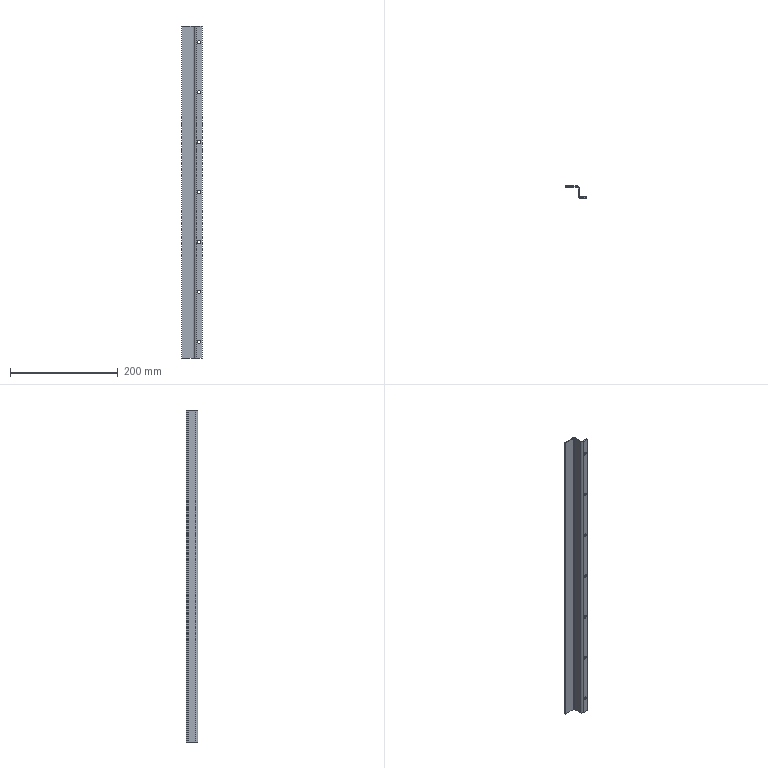Part | NX | features solid 2 | 1 solid | 28 faces | box 38 x 22 x 617 mm | volume 67998 mm3 | cylinder 18 | plane 10 | commonest cylinder face diameters 6 x14 4 x2 8 x2
STEP:
#1=CARTESIAN_POINT('',(1011.,-1578.,925.));
#2=VERTEX_POINT('',#1);
#3=CARTESIAN_POINT('',(1011.,-1576.,925.));
#4=VERTEX_POINT('',#3);
#5=CARTESIAN_POINT('',(1011.,-2194.56,925.));
#6=DIRECTION('',(0.,1.,0.));
#7=VECTOR('',#6,1000.);
#8=LINE('',#5,#7);
#9=EDGE_CURVE('',#2,#4,#8,.T.);
#10=ORIENTED_EDGE('',*,*,#9,.F.);
#11=CARTESIAN_POINT('',(1017.,-1578.,925.));
#12=VERTEX_POINT('',#11);
#13=CARTESIAN_POINT('',(1014.,-1578.,925.));
#14=DIRECTION('',(0.,1.,0.));
#15=DIRECTION('',(1.,0.,0.));
#16=AXIS2_PLACEMENT_3D('',#13,#14,#15);
#17=CIRCLE('',#16,3.);
#18=EDGE_CURVE('',#12,#2,#17,.T.);
#19=ORIENTED_EDGE('',*,*,#18,.F.);
#20=CARTESIAN_POINT('',(1017.,-1576.,925.));
#21=VERTEX_POINT('',#20);
#22=CARTESIAN_POINT('',(1017.,-2194.56,925.));
#23=DIRECTION('',(0.,1.,0.));
#24=VECTOR('',#23,1000.);
#25=LINE('',#22,#24);
#26=EDGE_CURVE('',#21,#12,#25,.F.);
#27=ORIENTED_EDGE('',*,*,#26,.F.);
#28=CARTESIAN_POINT('',(1014.,-1576.,925.));
#29=DIRECTION('',(0.,1.,0.));
#30=DIRECTION('',(0.,0.,1.));
#31=AXIS2_PLACEMENT_3D('',#28,#29,#30);
#32=CIRCLE('',#31,3.);
#33=EDGE_CURVE('',#21,#4,#32,.T.);
#34=ORIENTED_EDGE('',*,*,#33,.T.);
#35=EDGE_LOOP('',(#10,#19,#27,#34));
#36=FACE_BOUND('',#35,.T.);
#37=CARTESIAN_POINT('',(1014.,-2194.56,925.));
#38=DIRECTION('',(0.,1.,0.));
#39=DIRECTION('',(1.,0.,0.));
#40=AXIS2_PLACEMENT_3D('',#37,#38,#39);
#41=CYLINDRICAL_SURFACE('',#40,3.);
#42=ADVANCED_FACE('',(#36),#41,.F.);
#43=CARTESIAN_POINT('',(1011.,-1578.,832.167));
#44=VERTEX_POINT('',#43);
#45=CARTESIAN_POINT('',(1011.,-1576.,832.167));
#46=VERTEX_POINT('',#45);
#47=CARTESIAN_POINT('',(1011.,-2194.56,832.167));
#48=DIRECTION('',(0.,1.,0.));
#49=VECTOR('',#48,1000.);
#50=LINE('',#47,#49);
#51=EDGE_CURVE('',#44,#46,#50,.T.);
#52=ORIENTED_EDGE('',*,*,#51,.F.);
#53=CARTESIAN_POINT('',(1017.,-1578.,832.167));
#54=VERTEX_POINT('',#53);
#55=CARTESIAN_POINT('',(1014.,-1578.,832.167));
#56=DIRECTION('',(0.,1.,0.));
#57=DIRECTION('',(1.,0.,0.));
#58=AXIS2_PLACEMENT_3D('',#55,#56,#57);
#59=CIRCLE('',#58,3.);
#60=EDGE_CURVE('',#54,#44,#59,.T.);
#61=ORIENTED_EDGE('',*,*,#60,.F.);
#62=CARTESIAN_POINT('',(1017.,-1576.,832.167));
#63=VERTEX_POINT('',#62);
#64=CARTESIAN_POINT('',(1017.,-2194.56,832.167));
#65=DIRECTION('',(0.,1.,0.));
#66=VECTOR('',#65,1000.);
#67=LINE('',#64,#66);
#68=EDGE_CURVE('',#63,#54,#67,.F.);
#69=ORIENTED_EDGE('',*,*,#68,.F.);
#70=CARTESIAN_POINT('',(1014.,-1576.,832.167));
#71=DIRECTION('',(0.,1.,0.));
#72=DIRECTION('',(0.,0.,1.));
#73=AXIS2_PLACEMENT_3D('',#70,#71,#72);
#74=CIRCLE('',#73,3.);
#75=EDGE_CURVE('',#63,#46,#74,.T.);
#76=ORIENTED_EDGE('',*,*,#75,.T.);
#77=EDGE_LOOP('',(#52,#61,#69,#76));
#78=FACE_BOUND('',#77,.T.);
#79=CARTESIAN_POINT('',(1014.,-2194.56,832.167));
#80=DIRECTION('',(0.,1.,0.));
#81=DIRECTION('',(1.,0.,0.));
#82=AXIS2_PLACEMENT_3D('',#79,#80,#81);
#83=CYLINDRICAL_SURFACE('',#82,3.);
#84=ADVANCED_FACE('',(#78),#83,.F.);
#85=CARTESIAN_POINT('',(1011.,-1576.,739.333));
#86=VERTEX_POINT('',#85);
#87=CARTESIAN_POINT('',(1011.,-1578.,739.333));
#88=VERTEX_POINT('',#87);
#89=CARTESIAN_POINT('',(1011.,-2194.56,739.333));
#90=DIRECTION('',(0.,1.,0.));
#91=VECTOR('',#90,1000.);
#92=LINE('',#89,#91);
#93=EDGE_CURVE('',#86,#88,#92,.F.);
#94=ORIENTED_EDGE('',*,*,#93,.T.);
#95=CARTESIAN_POINT('',(1017.,-1578.,739.333));
#96=VERTEX_POINT('',#95);
#97=CARTESIAN_POINT('',(1014.,-1578.,739.333));
#98=DIRECTION('',(0.,1.,0.));
#99=DIRECTION('',(1.,0.,0.));
#100=AXIS2_PLACEMENT_3D('',#97,#98,#99);
#101=CIRCLE('',#100,3.);
#102=EDGE_CURVE('',#96,#88,#101,.T.);
#103=ORIENTED_EDGE('',*,*,#102,.F.);
#104=CARTESIAN_POINT('',(1017.,-1576.,739.333));
#105=VERTEX_POINT('',#104);
#106=CARTESIAN_POINT('',(1017.,-2194.56,739.333));
#107=DIRECTION('',(0.,1.,0.));
#108=VECTOR('',#107,1000.);
#109=LINE('',#106,#108);
#110=EDGE_CURVE('',#96,#105,#109,.T.);
#111=ORIENTED_EDGE('',*,*,#110,.T.);
#112=CARTESIAN_POINT('',(1014.,-1576.,739.333));
#113=DIRECTION('',(0.,1.,0.));
#114=DIRECTION('',(0.,0.,1.));
#115=AXIS2_PLACEMENT_3D('',#112,#113,#114);
#116=CIRCLE('',#115,3.);
#117=EDGE_CURVE('',#105,#86,#116,.T.);
#118=ORIENTED_EDGE('',*,*,#117,.T.);
#119=EDGE_LOOP('',(#94,#103,#111,#118));
#120=FACE_BOUND('',#119,.T.);
#121=CARTESIAN_POINT('',(1014.,-2194.56,739.333));
#122=DIRECTION('',(0.,1.,0.));
#123=DIRECTION('',(1.,0.,0.));
#124=AXIS2_PLACEMENT_3D('',#121,#122,#123);
#125=CYLINDRICAL_SURFACE('',#124,3.);
#126=ADVANCED_FACE('',(#120),#125,.F.);
#127=CARTESIAN_POINT('',(1011.,-1578.,646.5));
#128=VERTEX_POINT('',#127);
#129=CARTESIAN_POINT('',(1011.,-1576.,646.5));
#130=VERTEX_POINT('',#129);
#131=CARTESIAN_POINT('',(1011.,-2194.56,646.5));
#132=DIRECTION('',(0.,1.,0.));
#133=VECTOR('',#132,1000.);
#134=LINE('',#131,#133);
#135=EDGE_CURVE('',#128,#130,#134,.T.);
#136=ORIENTED_EDGE('',*,*,#135,.F.);
#137=CARTESIAN_POINT('',(1017.,-1578.,646.5));
#138=VERTEX_POINT('',#137);
#139=CARTESIAN_POINT('',(1014.,-1578.,646.5));
#140=DIRECTION('',(0.,1.,0.));
#141=DIRECTION('',(1.,0.,0.));
#142=AXIS2_PLACEMENT_3D('',#139,#140,#141);
#143=CIRCLE('',#142,3.);
#144=EDGE_CURVE('',#138,#128,#143,.T.);
#145=ORIENTED_EDGE('',*,*,#144,.F.);
#146=CARTESIAN_POINT('',(1017.,-1576.,646.5));
#147=VERTEX_POINT('',#146);
#148=CARTESIAN_POINT('',(1017.,-2194.56,646.5));
#149=DIRECTION('',(0.,1.,0.));
#150=VECTOR('',#149,1000.);
#151=LINE('',#148,#150);
#152=EDGE_CURVE('',#147,#138,#151,.F.);
#153=ORIENTED_EDGE('',*,*,#152,.F.);
#154=CARTESIAN_POINT('',(1014.,-1576.,646.5));
#155=DIRECTION('',(0.,1.,0.));
#156=DIRECTION('',(0.,0.,1.));
#157=AXIS2_PLACEMENT_3D('',#154,#155,#156);
#158=CIRCLE('',#157,3.);
#159=EDGE_CURVE('',#147,#130,#158,.T.);
#160=ORIENTED_EDGE('',*,*,#159,.T.);
#161=EDGE_LOOP('',(#136,#145,#153,#160));
#162=FACE_BOUND('',#161,.T.);
#163=CARTESIAN_POINT('',(1014.,-2194.56,646.5));
#164=DIRECTION('',(0.,1.,0.));
#165=DIRECTION('',(1.,0.,0.));
#166=AXIS2_PLACEMENT_3D('',#163,#164,#165);
#167=CYLINDRICAL_SURFACE('',#166,3.);
#168=ADVANCED_FACE('',(#162),#167,.F.);
#169=CARTESIAN_POINT('',(1011.,-1576.,553.667));
#170=VERTEX_POINT('',#169);
#171=CARTESIAN_POINT('',(1011.,-1578.,553.667));
#172=VERTEX_POINT('',#171);
#173=CARTESIAN_POINT('',(1011.,-2194.56,553.667));
#174=DIRECTION('',(0.,1.,0.));
#175=VECTOR('',#174,1000.);
#176=LINE('',#173,#175);
#177=EDGE_CURVE('',#170,#172,#176,.F.);
#178=ORIENTED_EDGE('',*,*,#177,.T.);
#179=CARTESIAN_POINT('',(1017.,-1578.,553.667));
#180=VERTEX_POINT('',#179);
#181=CARTESIAN_POINT('',(1014.,-1578.,553.667));
#182=DIRECTION('',(0.,1.,0.));
#183=DIRECTION('',(1.,0.,0.));
#184=AXIS2_PLACEMENT_3D('',#181,#182,#183);
#185=CIRCLE('',#184,3.);
#186=EDGE_CURVE('',#180,#172,#185,.T.);
#187=ORIENTED_EDGE('',*,*,#186,.F.);
#188=CARTESIAN_POINT('',(1017.,-1576.,553.667));
#189=VERTEX_POINT('',#188);
#190=CARTESIAN_POINT('',(1017.,-2194.56,553.667));
#191=DIRECTION('',(0.,1.,0.));
#192=VECTOR('',#191,1000.);
#193=LINE('',#190,#192);
#194=EDGE_CURVE('',#180,#189,#193,.T.);
#195=ORIENTED_EDGE('',*,*,#194,.T.);
#196=CARTESIAN_POINT('',(1014.,-1576.,553.667));
#197=DIRECTION('',(0.,1.,0.));
#198=DIRECTION('',(0.,0.,1.));
#199=AXIS2_PLACEMENT_3D('',#196,#197,#198);
#200=CIRCLE('',#199,3.);
#201=EDGE_CURVE('',#189,#170,#200,.T.);
#202=ORIENTED_EDGE('',*,*,#201,.T.);
#203=EDGE_LOOP('',(#178,#187,#195,#202));
#204=FACE_BOUND('',#203,.T.);
#205=CARTESIAN_POINT('',(1014.,-2194.56,553.667));
#206=DIRECTION('',(0.,1.,0.));
#207=DIRECTION('',(1.,0.,0.));
#208=AXIS2_PLACEMENT_3D('',#205,#206,#207);
#209=CYLINDRICAL_SURFACE('',#208,3.);
#210=ADVANCED_FACE('',(#204),#209,.F.);
#211=CARTESIAN_POINT('',(1011.,-1576.,460.833));
#212=VERTEX_POINT('',#211);
#213=CARTESIAN_POINT('',(1011.,-1578.,460.833));
#214=VERTEX_POINT('',#213);
#215=CARTESIAN_POINT('',(1011.,-2194.56,460.833));
#216=DIRECTION('',(0.,1.,0.));
#217=VECTOR('',#216,1000.);
#218=LINE('',#215,#217);
#219=EDGE_CURVE('',#212,#214,#218,.F.);
#220=ORIENTED_EDGE('',*,*,#219,.T.);
#221=CARTESIAN_POINT('',(1017.,-1578.,460.833));
#222=VERTEX_POINT('',#221);
#223=CARTESIAN_POINT('',(1014.,-1578.,460.833));
#224=DIRECTION('',(0.,1.,0.));
#225=DIRECTION('',(1.,0.,0.));
#226=AXIS2_PLACEMENT_3D('',#223,#224,#225);
#227=CIRCLE('',#226,3.);
#228=EDGE_CURVE('',#222,#214,#227,.T.);
#229=ORIENTED_EDGE('',*,*,#228,.F.);
#230=CARTESIAN_POINT('',(1017.,-1576.,460.833));
#231=VERTEX_POINT('',#230);
#232=CARTESIAN_POINT('',(1017.,-2194.56,460.833));
#233=DIRECTION('',(0.,1.,0.));
#234=VECTOR('',#233,1000.);
#235=LINE('',#232,#234);
#236=EDGE_CURVE('',#222,#231,#235,.T.);
#237=ORIENTED_EDGE('',*,*,#236,.T.);
#238=CARTESIAN_POINT('',(1014.,-1576.,460.833));
#239=DIRECTION('',(0.,1.,0.));
#240=DIRECTION('',(0.,0.,1.));
#241=AXIS2_PLACEMENT_3D('',#238,#239,#240);
#242=CIRCLE('',#241,3.);
#243=EDGE_CURVE('',#231,#212,#242,.T.);
#244=ORIENTED_EDGE('',*,*,#243,.T.);
#245=EDGE_LOOP('',(#220,#229,#237,#244));
#246=FACE_BOUND('',#245,.T.);
#247=CARTESIAN_POINT('',(1014.,-2194.56,460.833));
#248=DIRECTION('',(0.,1.,0.));
#249=DIRECTION('',(1.,0.,0.));
#250=AXIS2_PLACEMENT_3D('',#247,#248,#249);
#251=CYLINDRICAL_SURFACE('',#250,3.);
#252=ADVANCED_FACE('',(#246),#251,.F.);
#253=CARTESIAN_POINT('',(1011.,-1578.,368.));
#254=VERTEX_POINT('',#253);
#255=CARTESIAN_POINT('',(1011.,-1576.,368.));
#256=VERTEX_POINT('',#255);
#257=CARTESIAN_POINT('',(1011.,-2194.56,368.));
#258=DIRECTION('',(0.,1.,0.));
#259=VECTOR('',#258,1000.);
#260=LINE('',#257,#259);
#261=EDGE_CURVE('',#254,#256,#260,.T.);
#262=ORIENTED_EDGE('',*,*,#261,.F.);
#263=CARTESIAN_POINT('',(1017.,-1578.,368.));
#264=VERTEX_POINT('',#263);
#265=CARTESIAN_POINT('',(1014.,-1578.,368.));
#266=DIRECTION('',(0.,1.,0.));
#267=DIRECTION('',(1.,0.,0.));
#268=AXIS2_PLACEMENT_3D('',#265,#266,#267);
#269=CIRCLE('',#268,3.);
#270=EDGE_CURVE('',#264,#254,#269,.T.);
#271=ORIENTED_EDGE('',*,*,#270,.F.);
#272=CARTESIAN_POINT('',(1017.,-1576.,368.));
#273=VERTEX_POINT('',#272);
#274=CARTESIAN_POINT('',(1017.,-2194.56,368.));
#275=DIRECTION('',(0.,1.,0.));
#276=VECTOR('',#275,1000.);
#277=LINE('',#274,#276);
#278=EDGE_CURVE('',#273,#264,#277,.F.);
#279=ORIENTED_EDGE('',*,*,#278,.F.);
#280=CARTESIAN_POINT('',(1014.,-1576.,368.));
#281=DIRECTION('',(0.,1.,0.));
#282=DIRECTION('',(0.,0.,1.));
#283=AXIS2_PLACEMENT_3D('',#280,#281,#282);
#284=CIRCLE('',#283,3.);
#285=EDGE_CURVE('',#273,#256,#284,.T.);
#286=ORIENTED_EDGE('',*,*,#285,.T.);
#287=EDGE_LOOP('',(#262,#271,#279,#286));
#288=FACE_BOUND('',#287,.T.);
#289=CARTESIAN_POINT('',(1014.,-2194.56,368.));
#290=DIRECTION('',(0.,1.,0.));
#291=DIRECTION('',(1.,0.,0.));
#292=AXIS2_PLACEMENT_3D('',#289,#290,#291);
#293=CYLINDRICAL_SURFACE('',#292,3.);
#294=ADVANCED_FACE('',(#288),#293,.F.);
#295=CARTESIAN_POINT('',(1003.,-1558.,955.));
#296=VERTEX_POINT('',#295);
#297=CARTESIAN_POINT('',(982.,-1558.,955.));
#298=VERTEX_POINT('',#297);
#299=CARTESIAN_POINT('',(1005.,-1558.,955.));
#300=DIRECTION('',(-1.,0.,0.));
#301=VECTOR('',#300,1000.);
#302=LINE('',#299,#301);
#303=EDGE_CURVE('',#296,#298,#302,.T.);
#304=ORIENTED_EDGE('',*,*,#303,.T.);
#305=CARTESIAN_POINT('',(982.,-1558.,338.));
#306=VERTEX_POINT('',#305);
#307=CARTESIAN_POINT('',(982.,-1558.,338.));
#308=DIRECTION('',(0.,0.,1.));
#309=VECTOR('',#308,1000.);
#310=LINE('',#307,#309);
#311=EDGE_CURVE('',#306,#298,#310,.T.);
#312=ORIENTED_EDGE('',*,*,#311,.F.);
#313=CARTESIAN_POINT('',(1003.,-1558.,338.));
#314=VERTEX_POINT('',#313);
#315=CARTESIAN_POINT('',(1005.,-1558.,338.));
#316=DIRECTION('',(-1.,0.,0.));
#317=VECTOR('',#316,1000.);
#318=LINE('',#315,#317);
#319=EDGE_CURVE('',#314,#306,#318,.T.);
#320=ORIENTED_EDGE('',*,*,#319,.F.);
#321=CARTESIAN_POINT('',(1003.,-1558.,338.));
#322=DIRECTION('',(0.,0.,1.));
#323=VECTOR('',#322,1000.);
#324=LINE('',#321,#323);
#325=EDGE_CURVE('',#314,#296,#324,.T.);
#326=ORIENTED_EDGE('',*,*,#325,.T.);
#327=EDGE_LOOP('',(#304,#312,#320,#326));
#328=FACE_BOUND('',#327,.T.);
#329=CARTESIAN_POINT('',(1005.,-1558.,338.));
#330=DIRECTION('',(0.,1.,0.));
#331=DIRECTION('',(0.,0.,-1.));
#332=AXIS2_PLACEMENT_3D('',#329,#330,#331);
#333=PLANE('',#332);
#334=ADVANCED_FACE('',(#328),#333,.F.);
#335=CARTESIAN_POINT('',(1005.,-1560.,955.));
#336=VERTEX_POINT('',#335);
#337=CARTESIAN_POINT('',(1003.,-1560.,955.));
#338=DIRECTION('',(0.,0.,1.));
#339=DIRECTION('',(1.,0.,0.));
#340=AXIS2_PLACEMENT_3D('',#337,#338,#339);
#341=CIRCLE('',#340,2.);
#342=EDGE_CURVE('',#336,#296,#341,.T.);
#343=ORIENTED_EDGE('',*,*,#342,.T.);
#344=ORIENTED_EDGE('',*,*,#325,.F.);
#345=CARTESIAN_POINT('',(1005.,-1560.,338.));
#346=VERTEX_POINT('',#345);
#347=CARTESIAN_POINT('',(1003.,-1560.,338.));
#348=DIRECTION('',(0.,0.,1.));
#349=DIRECTION('',(1.,0.,0.));
#350=AXIS2_PLACEMENT_3D('',#347,#348,#349);
#351=CIRCLE('',#350,2.);
#352=EDGE_CURVE('',#346,#314,#351,.T.);
#353=ORIENTED_EDGE('',*,*,#352,.F.);
#354=CARTESIAN_POINT('',(1005.,-1560.,338.));
#355=DIRECTION('',(0.,0.,1.));
#356=VECTOR('',#355,1000.);
#357=LINE('',#354,#356);
#358=EDGE_CURVE('',#346,#336,#357,.T.);
#359=ORIENTED_EDGE('',*,*,#358,.T.);
#360=EDGE_LOOP('',(#343,#344,#353,#359));
#361=FACE_BOUND('',#360,.T.);
#362=CARTESIAN_POINT('',(1003.,-1560.,338.));
#363=DIRECTION('',(0.,0.,1.));
#364=DIRECTION('',(-1.,0.,0.));
#365=AXIS2_PLACEMENT_3D('',#362,#363,#364);
#366=CYLINDRICAL_SURFACE('',#365,2.);
#367=ADVANCED_FACE('',(#361),#366,.F.);
#368=CARTESIAN_POINT('',(1005.,-1574.,955.));
#369=VERTEX_POINT('',#368);
#370=CARTESIAN_POINT('',(1005.,-1578.,955.));
#371=DIRECTION('',(0.,1.,0.));
#372=VECTOR('',#371,1000.);
#373=LINE('',#370,#372);
#374=EDGE_CURVE('',#369,#336,#373,.T.);
#375=ORIENTED_EDGE('',*,*,#374,.T.);
#376=ORIENTED_EDGE('',*,*,#358,.F.);
#377=CARTESIAN_POINT('',(1005.,-1574.,338.));
#378=VERTEX_POINT('',#377);
#379=CARTESIAN_POINT('',(1005.,-1578.,338.));
#380=DIRECTION('',(0.,1.,0.));
#381=VECTOR('',#380,1000.);
#382=LINE('',#379,#381);
#383=EDGE_CURVE('',#378,#346,#382,.T.);
#384=ORIENTED_EDGE('',*,*,#383,.F.);
#385=CARTESIAN_POINT('',(1005.,-1574.,338.));
#386=DIRECTION('',(0.,0.,1.));
#387=VECTOR('',#386,1000.);
#388=LINE('',#385,#387);
#389=EDGE_CURVE('',#378,#369,#388,.T.);
#390=ORIENTED_EDGE('',*,*,#389,.T.);
#391=EDGE_LOOP('',(#375,#376,#384,#390));
#392=FACE_BOUND('',#391,.T.);
#393=CARTESIAN_POINT('',(1005.,-1578.,338.));
#394=DIRECTION('',(1.,0.,0.));
#395=DIRECTION('',(0.,0.,-1.));
#396=AXIS2_PLACEMENT_3D('',#393,#394,#395);
#397=PLANE('',#396);
#398=ADVANCED_FACE('',(#392),#397,.F.);
#399=CARTESIAN_POINT('',(1009.,-1578.,955.));
#400=VERTEX_POINT('',#399);
#401=CARTESIAN_POINT('',(1009.,-1574.,955.));
#402=DIRECTION('',(0.,0.,-1.));
#403=DIRECTION('',(-1.,0.,0.));
#404=AXIS2_PLACEMENT_3D('',#401,#402,#403);
#405=CIRCLE('',#404,4.);
#406=EDGE_CURVE('',#400,#369,#405,.T.);
#407=ORIENTED_EDGE('',*,*,#406,.T.);
#408=ORIENTED_EDGE('',*,*,#389,.F.);
#409=CARTESIAN_POINT('',(1009.,-1578.,338.));
#410=VERTEX_POINT('',#409);
#411=CARTESIAN_POINT('',(1009.,-1574.,338.));
#412=DIRECTION('',(0.,0.,-1.));
#413=DIRECTION('',(-1.,0.,0.));
#414=AXIS2_PLACEMENT_3D('',#411,#412,#413);
#415=CIRCLE('',#414,4.);
#416=EDGE_CURVE('',#410,#378,#415,.T.);
#417=ORIENTED_EDGE('',*,*,#416,.F.);
#418=CARTESIAN_POINT('',(1009.,-1578.,338.));
#419=DIRECTION('',(0.,0.,1.));
#420=VECTOR('',#419,1000.);
#421=LINE('',#418,#420);
#422=EDGE_CURVE('',#410,#400,#421,.T.);
#423=ORIENTED_EDGE('',*,*,#422,.T.);
#424=EDGE_LOOP('',(#407,#408,#417,#423));
#425=FACE_BOUND('',#424,.T.);
#426=CARTESIAN_POINT('',(1009.,-1574.,338.));
#427=DIRECTION('',(0.,0.,1.));
#428=DIRECTION('',(-1.,0.,0.));
#429=AXIS2_PLACEMENT_3D('',#426,#427,#428);
#430=CYLINDRICAL_SURFACE('',#429,4.);
#431=ADVANCED_FACE('',(#425),#430,.T.);
#432=ORIENTED_EDGE('',*,*,#270,.T.);
#433=CARTESIAN_POINT('',(1014.,-1578.,368.));
#434=DIRECTION('',(0.,1.,0.));
#435=DIRECTION('',(1.,0.,0.));
#436=AXIS2_PLACEMENT_3D('',#433,#434,#435);
#437=CIRCLE('',#436,3.);
#438=EDGE_CURVE('',#254,#264,#437,.T.);
#439=ORIENTED_EDGE('',*,*,#438,.T.);
#440=EDGE_LOOP('',(#432,#439));
#441=FACE_BOUND('',#440,.T.);
#442=ORIENTED_EDGE('',*,*,#228,.T.);
#443=CARTESIAN_POINT('',(1014.,-1578.,460.833));
#444=DIRECTION('',(0.,1.,0.));
#445=DIRECTION('',(1.,0.,0.));
#446=AXIS2_PLACEMENT_3D('',#443,#444,#445);
#447=CIRCLE('',#446,3.);
#448=EDGE_CURVE('',#214,#222,#447,.T.);
#449=ORIENTED_EDGE('',*,*,#448,.T.);
#450=EDGE_LOOP('',(#442,#449));
#451=FACE_BOUND('',#450,.T.);
#452=ORIENTED_EDGE('',*,*,#186,.T.);
#453=CARTESIAN_POINT('',(1014.,-1578.,553.667));
#454=DIRECTION('',(0.,1.,0.));
#455=DIRECTION('',(1.,0.,0.));
#456=AXIS2_PLACEMENT_3D('',#453,#454,#455);
#457=CIRCLE('',#456,3.);
#458=EDGE_CURVE('',#172,#180,#457,.T.);
#459=ORIENTED_EDGE('',*,*,#458,.T.);
#460=EDGE_LOOP('',(#452,#459));
#461=FACE_BOUND('',#460,.T.);
#462=ORIENTED_EDGE('',*,*,#144,.T.);
#463=CARTESIAN_POINT('',(1014.,-1578.,646.5));
#464=DIRECTION('',(0.,1.,0.));
#465=DIRECTION('',(1.,0.,0.));
#466=AXIS2_PLACEMENT_3D('',#463,#464,#465);
#467=CIRCLE('',#466,3.);
#468=EDGE_CURVE('',#128,#138,#467,.T.);
#469=ORIENTED_EDGE('',*,*,#468,.T.);
#470=EDGE_LOOP('',(#462,#469));
#471=FACE_BOUND('',#470,.T.);
#472=ORIENTED_EDGE('',*,*,#102,.T.);
#473=CARTESIAN_POINT('',(1014.,-1578.,739.333));
#474=DIRECTION('',(0.,1.,0.));
#475=DIRECTION('',(1.,0.,0.));
#476=AXIS2_PLACEMENT_3D('',#473,#474,#475);
#477=CIRCLE('',#476,3.);
#478=EDGE_CURVE('',#88,#96,#477,.T.);
#479=ORIENTED_EDGE('',*,*,#478,.T.);
#480=EDGE_LOOP('',(#472,#479));
#481=FACE_BOUND('',#480,.T.);
#482=ORIENTED_EDGE('',*,*,#60,.T.);
#483=CARTESIAN_POINT('',(1014.,-1578.,832.167));
#484=DIRECTION('',(0.,1.,0.));
#485=DIRECTION('',(1.,0.,0.));
#486=AXIS2_PLACEMENT_3D('',#483,#484,#485);
#487=CIRCLE('',#486,3.);
#488=EDGE_CURVE('',#44,#54,#487,.T.);
#489=ORIENTED_EDGE('',*,*,#488,.T.);
#490=EDGE_LOOP('',(#482,#489));
#491=FACE_BOUND('',#490,.T.);
#492=ORIENTED_EDGE('',*,*,#18,.T.);
#493=CARTESIAN_POINT('',(1014.,-1578.,925.));
#494=DIRECTION('',(0.,1.,0.));
#495=DIRECTION('',(1.,0.,0.));
#496=AXIS2_PLACEMENT_3D('',#493,#494,#495);
#497=CIRCLE('',#496,3.);
#498=EDGE_CURVE('',#2,#12,#497,.T.);
#499=ORIENTED_EDGE('',*,*,#498,.T.);
#500=EDGE_LOOP('',(#492,#499));
#501=FACE_BOUND('',#500,.T.);
#502=CARTESIAN_POINT('',(1020.,-1578.,955.));
#503=VERTEX_POINT('',#502);
#504=CARTESIAN_POINT('',(1020.,-1578.,955.));
#505=DIRECTION('',(-1.,0.,0.));
#506=VECTOR('',#505,1000.);
#507=LINE('',#504,#506);
#508=EDGE_CURVE('',#503,#400,#507,.T.);
#509=ORIENTED_EDGE('',*,*,#508,.T.);
#510=ORIENTED_EDGE('',*,*,#422,.F.);
#511=CARTESIAN_POINT('',(1020.,-1578.,338.));
#512=VERTEX_POINT('',#511);
#513=CARTESIAN_POINT('',(1020.,-1578.,338.));
#514=DIRECTION('',(-1.,0.,0.));
#515=VECTOR('',#514,1000.);
#516=LINE('',#513,#515);
#517=EDGE_CURVE('',#512,#410,#516,.T.);
#518=ORIENTED_EDGE('',*,*,#517,.F.);
#519=CARTESIAN_POINT('',(1020.,-1578.,338.));
#520=DIRECTION('',(0.,0.,1.));
#521=VECTOR('',#520,1000.);
#522=LINE('',#519,#521);
#523=EDGE_CURVE('',#512,#503,#522,.T.);
#524=ORIENTED_EDGE('',*,*,#523,.T.);
#525=EDGE_LOOP('',(#509,#510,#518,#524));
#526=FACE_BOUND('',#525,.T.);
#527=CARTESIAN_POINT('',(1020.,-1578.,338.));
#528=DIRECTION('',(0.,1.,0.));
#529=DIRECTION('',(0.,0.,-1.));
#530=AXIS2_PLACEMENT_3D('',#527,#528,#529);
#531=PLANE('',#530);
#532=ADVANCED_FACE('',(#441,#451,#461,#471,#481,#491,#501,#526),#531,.F.);
#533=CARTESIAN_POINT('',(1003.,-1556.,955.));
#534=VERTEX_POINT('',#533);
#535=CARTESIAN_POINT('',(982.,-1556.,955.));
#536=VERTEX_POINT('',#535);
#537=CARTESIAN_POINT('',(1005.,-1556.,955.));
#538=DIRECTION('',(-1.,0.,0.));
#539=VECTOR('',#538,1000.);
#540=LINE('',#537,#539);
#541=EDGE_CURVE('',#534,#536,#540,.T.);
#542=ORIENTED_EDGE('',*,*,#541,.F.);
#543=CARTESIAN_POINT('',(1003.,-1556.,338.));
#544=VERTEX_POINT('',#543);
#545=CARTESIAN_POINT('',(1003.,-1556.,338.));
#546=DIRECTION('',(0.,0.,1.));
#547=VECTOR('',#546,1000.);
#548=LINE('',#545,#547);
#549=EDGE_CURVE('',#544,#534,#548,.T.);
#550=ORIENTED_EDGE('',*,*,#549,.F.);
#551=CARTESIAN_POINT('',(982.,-1556.,338.));
#552=VERTEX_POINT('',#551);
#553=CARTESIAN_POINT('',(1005.,-1556.,338.));
#554=DIRECTION('',(-1.,0.,0.));
#555=VECTOR('',#554,1000.);
#556=LINE('',#553,#555);
#557=EDGE_CURVE('',#544,#552,#556,.T.);
#558=ORIENTED_EDGE('',*,*,#557,.T.);
#559=CARTESIAN_POINT('',(982.,-1556.,338.));
#560=DIRECTION('',(0.,0.,1.));
#561=VECTOR('',#560,1000.);
#562=LINE('',#559,#561);
#563=EDGE_CURVE('',#552,#536,#562,.T.);
#564=ORIENTED_EDGE('',*,*,#563,.T.);
#565=EDGE_LOOP('',(#542,#550,#558,#564));
#566=FACE_BOUND('',#565,.T.);
#567=CARTESIAN_POINT('',(1005.,-1556.,338.));
#568=DIRECTION('',(0.,1.,0.));
#569=DIRECTION('',(0.,0.,-1.));
#570=AXIS2_PLACEMENT_3D('',#567,#568,#569);
#571=PLANE('',#570);
#572=ADVANCED_FACE('',(#566),#571,.T.);
#573=CARTESIAN_POINT('',(1007.,-1560.,955.));
#574=VERTEX_POINT('',#573);
#575=CARTESIAN_POINT('',(1003.,-1560.,955.));
#576=DIRECTION('',(0.,0.,1.));
#577=DIRECTION('',(-1.,0.,0.));
#578=AXIS2_PLACEMENT_3D('',#575,#576,#577);
#579=CIRCLE('',#578,4.);
#580=EDGE_CURVE('',#574,#534,#579,.T.);
#581=ORIENTED_EDGE('',*,*,#580,.F.);
#582=CARTESIAN_POINT('',(1007.,-1560.,338.));
#583=VERTEX_POINT('',#582);
#584=CARTESIAN_POINT('',(1007.,-1560.,338.));
#585=DIRECTION('',(0.,0.,1.));
#586=VECTOR('',#585,1000.);
#587=LINE('',#584,#586);
#588=EDGE_CURVE('',#583,#574,#587,.T.);
#589=ORIENTED_EDGE('',*,*,#588,.F.);
#590=CARTESIAN_POINT('',(1003.,-1560.,338.));
#591=DIRECTION('',(0.,0.,1.));
#592=DIRECTION('',(-1.,0.,0.));
#593=AXIS2_PLACEMENT_3D('',#590,#591,#592);
#594=CIRCLE('',#593,4.);
#595=EDGE_CURVE('',#583,#544,#594,.T.);
#596=ORIENTED_EDGE('',*,*,#595,.T.);
#597=ORIENTED_EDGE('',*,*,#549,.T.);
#598=EDGE_LOOP('',(#581,#589,#596,#597));
#599=FACE_BOUND('',#598,.T.);
#600=CARTESIAN_POINT('',(1003.,-1560.,338.));
#601=DIRECTION('',(0.,0.,1.));
#602=DIRECTION('',(-1.,0.,0.));
#603=AXIS2_PLACEMENT_3D('',#600,#601,#602);
#604=CYLINDRICAL_SURFACE('',#603,4.);
#605=ADVANCED_FACE('',(#599),#604,.T.);
#606=CARTESIAN_POINT('',(1007.,-1574.,955.));
#607=VERTEX_POINT('',#606);
#608=CARTESIAN_POINT('',(1007.,-1578.,955.));
#609=DIRECTION('',(0.,1.,0.));
#610=VECTOR('',#609,1000.);
#611=LINE('',#608,#610);
#612=EDGE_CURVE('',#607,#574,#611,.T.);
#613=ORIENTED_EDGE('',*,*,#612,.F.);
#614=CARTESIAN_POINT('',(1007.,-1574.,338.));
#615=VERTEX_POINT('',#614);
#616=CARTESIAN_POINT('',(1007.,-1574.,338.));
#617=DIRECTION('',(0.,0.,1.));
#618=VECTOR('',#617,1000.);
#619=LINE('',#616,#618);
#620=EDGE_CURVE('',#615,#607,#619,.T.);
#621=ORIENTED_EDGE('',*,*,#620,.F.);
#622=CARTESIAN_POINT('',(1007.,-1578.,338.));
#623=DIRECTION('',(0.,1.,0.));
#624=VECTOR('',#623,1000.);
#625=LINE('',#622,#624);
#626=EDGE_CURVE('',#615,#583,#625,.T.);
#627=ORIENTED_EDGE('',*,*,#626,.T.);
#628=ORIENTED_EDGE('',*,*,#588,.T.);
#629=EDGE_LOOP('',(#613,#621,#627,#628));
#630=FACE_BOUND('',#629,.T.);
#631=CARTESIAN_POINT('',(1007.,-1578.,338.));
#632=DIRECTION('',(1.,0.,0.));
#633=DIRECTION('',(0.,0.,-1.));
#634=AXIS2_PLACEMENT_3D('',#631,#632,#633);
#635=PLANE('',#634);
#636=ADVANCED_FACE('',(#630),#635,.T.);
#637=CARTESIAN_POINT('',(1009.,-1576.,955.));
#638=VERTEX_POINT('',#637);
#639=CARTESIAN_POINT('',(1009.,-1574.,955.));
#640=DIRECTION('',(0.,0.,-1.));
#641=DIRECTION('',(-1.,0.,0.));
#642=AXIS2_PLACEMENT_3D('',#639,#640,#641);
#643=CIRCLE('',#642,2.);
#644=EDGE_CURVE('',#638,#607,#643,.T.);
#645=ORIENTED_EDGE('',*,*,#644,.F.);
#646=CARTESIAN_POINT('',(1009.,-1576.,338.));
#647=VERTEX_POINT('',#646);
#648=CARTESIAN_POINT('',(1009.,-1576.,338.));
#649=DIRECTION('',(0.,0.,1.));
#650=VECTOR('',#649,1000.);
#651=LINE('',#648,#650);
#652=EDGE_CURVE('',#647,#638,#651,.T.);
#653=ORIENTED_EDGE('',*,*,#652,.F.);
#654=CARTESIAN_POINT('',(1009.,-1574.,338.));
#655=DIRECTION('',(0.,0.,-1.));
#656=DIRECTION('',(-1.,0.,0.));
#657=AXIS2_PLACEMENT_3D('',#654,#655,#656);
#658=CIRCLE('',#657,2.);
#659=EDGE_CURVE('',#647,#615,#658,.T.);
#660=ORIENTED_EDGE('',*,*,#659,.T.);
#661=ORIENTED_EDGE('',*,*,#620,.T.);
#662=EDGE_LOOP('',(#645,#653,#660,#661));
#663=FACE_BOUND('',#662,.T.);
#664=CARTESIAN_POINT('',(1009.,-1574.,338.));
#665=DIRECTION('',(0.,0.,1.));
#666=DIRECTION('',(-1.,0.,0.));
#667=AXIS2_PLACEMENT_3D('',#664,#665,#666);
#668=CYLINDRICAL_SURFACE('',#667,2.);
#669=ADVANCED_FACE('',(#663),#668,.F.);
#670=ORIENTED_EDGE('',*,*,#285,.F.);
#671=CARTESIAN_POINT('',(1014.,-1576.,368.));
#672=DIRECTION('',(0.,1.,0.));
#673=DIRECTION('',(0.,0.,1.));
#674=AXIS2_PLACEMENT_3D('',#671,#672,#673);
#675=CIRCLE('',#674,3.);
#676=EDGE_CURVE('',#256,#273,#675,.T.);
#677=ORIENTED_EDGE('',*,*,#676,.F.);
#678=EDGE_LOOP('',(#670,#677));
#679=FACE_BOUND('',#678,.T.);
#680=ORIENTED_EDGE('',*,*,#243,.F.);
#681=CARTESIAN_POINT('',(1014.,-1576.,460.833));
#682=DIRECTION('',(0.,1.,0.));
#683=DIRECTION('',(0.,0.,1.));
#684=AXIS2_PLACEMENT_3D('',#681,#682,#683);
#685=CIRCLE('',#684,3.);
#686=EDGE_CURVE('',#212,#231,#685,.T.);
#687=ORIENTED_EDGE('',*,*,#686,.F.);
#688=EDGE_LOOP('',(#680,#687));
#689=FACE_BOUND('',#688,.T.);
#690=ORIENTED_EDGE('',*,*,#201,.F.);
#691=CARTESIAN_POINT('',(1014.,-1576.,553.667));
#692=DIRECTION('',(0.,1.,0.));
#693=DIRECTION('',(0.,0.,1.));
#694=AXIS2_PLACEMENT_3D('',#691,#692,#693);
#695=CIRCLE('',#694,3.);
#696=EDGE_CURVE('',#170,#189,#695,.T.);
#697=ORIENTED_EDGE('',*,*,#696,.F.);
#698=EDGE_LOOP('',(#690,#697));
#699=FACE_BOUND('',#698,.T.);
#700=ORIENTED_EDGE('',*,*,#159,.F.);
#701=CARTESIAN_POINT('',(1014.,-1576.,646.5));
#702=DIRECTION('',(0.,1.,0.));
#703=DIRECTION('',(0.,0.,1.));
#704=AXIS2_PLACEMENT_3D('',#701,#702,#703);
#705=CIRCLE('',#704,3.);
#706=EDGE_CURVE('',#130,#147,#705,.T.);
#707=ORIENTED_EDGE('',*,*,#706,.F.);
#708=EDGE_LOOP('',(#700,#707));
#709=FACE_BOUND('',#708,.T.);
#710=ORIENTED_EDGE('',*,*,#117,.F.);
#711=CARTESIAN_POINT('',(1014.,-1576.,739.333));
#712=DIRECTION('',(0.,1.,0.));
#713=DIRECTION('',(0.,0.,1.));
#714=AXIS2_PLACEMENT_3D('',#711,#712,#713);
#715=CIRCLE('',#714,3.);
#716=EDGE_CURVE('',#86,#105,#715,.T.);
#717=ORIENTED_EDGE('',*,*,#716,.F.);
#718=EDGE_LOOP('',(#710,#717));
#719=FACE_BOUND('',#718,.T.);
#720=ORIENTED_EDGE('',*,*,#75,.F.);
#721=CARTESIAN_POINT('',(1014.,-1576.,832.167));
#722=DIRECTION('',(0.,1.,0.));
#723=DIRECTION('',(0.,0.,1.));
#724=AXIS2_PLACEMENT_3D('',#721,#722,#723);
#725=CIRCLE('',#724,3.);
#726=EDGE_CURVE('',#46,#63,#725,.T.);
#727=ORIENTED_EDGE('',*,*,#726,.F.);
#728=EDGE_LOOP('',(#720,#727));
#729=FACE_BOUND('',#728,.T.);
#730=ORIENTED_EDGE('',*,*,#33,.F.);
#731=CARTESIAN_POINT('',(1014.,-1576.,925.));
#732=DIRECTION('',(0.,1.,0.));
#733=DIRECTION('',(0.,0.,1.));
#734=AXIS2_PLACEMENT_3D('',#731,#732,#733);
#735=CIRCLE('',#734,3.);
#736=EDGE_CURVE('',#4,#21,#735,.T.);
#737=ORIENTED_EDGE('',*,*,#736,.F.);
#738=EDGE_LOOP('',(#730,#737));
#739=FACE_BOUND('',#738,.T.);
#740=CARTESIAN_POINT('',(1020.,-1576.,955.));
#741=VERTEX_POINT('',#740);
#742=CARTESIAN_POINT('',(1020.,-1576.,955.));
#743=DIRECTION('',(-1.,0.,0.));
#744=VECTOR('',#743,1000.);
#745=LINE('',#742,#744);
#746=EDGE_CURVE('',#741,#638,#745,.T.);
#747=ORIENTED_EDGE('',*,*,#746,.F.);
#748=CARTESIAN_POINT('',(1020.,-1576.,338.));
#749=VERTEX_POINT('',#748);
#750=CARTESIAN_POINT('',(1020.,-1576.,338.));
#751=DIRECTION('',(0.,0.,1.));
#752=VECTOR('',#751,1000.);
#753=LINE('',#750,#752);
#754=EDGE_CURVE('',#749,#741,#753,.T.);
#755=ORIENTED_EDGE('',*,*,#754,.F.);
#756=CARTESIAN_POINT('',(1020.,-1576.,338.));
#757=DIRECTION('',(-1.,0.,0.));
#758=VECTOR('',#757,1000.);
#759=LINE('',#756,#758);
#760=EDGE_CURVE('',#749,#647,#759,.T.);
#761=ORIENTED_EDGE('',*,*,#760,.T.);
#762=ORIENTED_EDGE('',*,*,#652,.T.);
#763=EDGE_LOOP('',(#747,#755,#761,#762));
#764=FACE_BOUND('',#763,.T.);
#765=CARTESIAN_POINT('',(1020.,-1576.,338.));
#766=DIRECTION('',(0.,1.,0.));
#767=DIRECTION('',(0.,0.,-1.));
#768=AXIS2_PLACEMENT_3D('',#765,#766,#767);
#769=PLANE('',#768);
#770=ADVANCED_FACE('',(#679,#689,#699,#709,#719,#729,#739,#764),#769,.T.);
#771=ORIENTED_EDGE('',*,*,#523,.F.);
#772=CARTESIAN_POINT('',(1020.,-1578.,338.));
#773=DIRECTION('',(0.,1.,0.));
#774=VECTOR('',#773,1000.);
#775=LINE('',#772,#774);
#776=EDGE_CURVE('',#512,#749,#775,.T.);
#777=ORIENTED_EDGE('',*,*,#776,.T.);
#778=ORIENTED_EDGE('',*,*,#754,.T.);
#779=CARTESIAN_POINT('',(1020.,-1578.,955.));
#780=DIRECTION('',(0.,1.,0.));
#781=VECTOR('',#780,1000.);
#782=LINE('',#779,#781);
#783=EDGE_CURVE('',#503,#741,#782,.T.);
#784=ORIENTED_EDGE('',*,*,#783,.F.);
#785=EDGE_LOOP('',(#771,#777,#778,#784));
#786=FACE_BOUND('',#785,.T.);
#787=CARTESIAN_POINT('',(1020.,-1578.,338.));
#788=DIRECTION('',(-1.,0.,0.));
#789=DIRECTION('',(0.,1.,0.));
#790=AXIS2_PLACEMENT_3D('',#787,#788,#789);
#791=PLANE('',#790);
#792=ADVANCED_FACE('',(#786),#791,.F.);
#793=ORIENTED_EDGE('',*,*,#746,.T.);
#794=ORIENTED_EDGE('',*,*,#644,.T.);
#795=ORIENTED_EDGE('',*,*,#612,.T.);
#796=ORIENTED_EDGE('',*,*,#580,.T.);
#797=ORIENTED_EDGE('',*,*,#541,.T.);
#798=CARTESIAN_POINT('',(982.,-1558.,955.));
#799=DIRECTION('',(0.,1.,0.));
#800=VECTOR('',#799,1000.);
#801=LINE('',#798,#800);
#802=EDGE_CURVE('',#298,#536,#801,.T.);
#803=ORIENTED_EDGE('',*,*,#802,.F.);
#804=ORIENTED_EDGE('',*,*,#303,.F.);
#805=ORIENTED_EDGE('',*,*,#342,.F.);
#806=ORIENTED_EDGE('',*,*,#374,.F.);
#807=ORIENTED_EDGE('',*,*,#406,.F.);
#808=ORIENTED_EDGE('',*,*,#508,.F.);
#809=ORIENTED_EDGE('',*,*,#783,.T.);
#810=EDGE_LOOP('',(#793,#794,#795,#796,#797,#803,#804,#805,#806,#807,#808,#809));
#811=FACE_BOUND('',#810,.T.);
#812=CARTESIAN_POINT('',(1020.,-1578.,955.));
#813=DIRECTION('',(0.,0.,-1.));
#814=DIRECTION('',(0.,-1.,0.));
#815=AXIS2_PLACEMENT_3D('',#812,#813,#814);
#816=PLANE('',#815);
#817=ADVANCED_FACE('',(#811),#816,.F.);
#818=CARTESIAN_POINT('',(982.,-1558.,338.));
#819=DIRECTION('',(0.,1.,0.));
#820=VECTOR('',#819,1000.);
#821=LINE('',#818,#820);
#822=EDGE_CURVE('',#306,#552,#821,.T.);
#823=ORIENTED_EDGE('',*,*,#822,.F.);
#824=ORIENTED_EDGE('',*,*,#311,.T.);
#825=ORIENTED_EDGE('',*,*,#802,.T.);
#826=ORIENTED_EDGE('',*,*,#563,.F.);
#827=EDGE_LOOP('',(#823,#824,#825,#826));
#828=FACE_BOUND('',#827,.T.);
#829=CARTESIAN_POINT('',(982.,-1558.,338.));
#830=DIRECTION('',(-1.,0.,0.));
#831=DIRECTION('',(0.,1.,0.));
#832=AXIS2_PLACEMENT_3D('',#829,#830,#831);
#833=PLANE('',#832);
#834=ADVANCED_FACE('',(#828),#833,.T.);
#835=ORIENTED_EDGE('',*,*,#557,.F.);
#836=ORIENTED_EDGE('',*,*,#595,.F.);
#837=ORIENTED_EDGE('',*,*,#626,.F.);
#838=ORIENTED_EDGE('',*,*,#659,.F.);
#839=ORIENTED_EDGE('',*,*,#760,.F.);
#840=ORIENTED_EDGE('',*,*,#776,.F.);
#841=ORIENTED_EDGE('',*,*,#517,.T.);
#842=ORIENTED_EDGE('',*,*,#416,.T.);
#843=ORIENTED_EDGE('',*,*,#383,.T.);
#844=ORIENTED_EDGE('',*,*,#352,.T.);
#845=ORIENTED_EDGE('',*,*,#319,.T.);
#846=ORIENTED_EDGE('',*,*,#822,.T.);
#847=EDGE_LOOP('',(#835,#836,#837,#838,#839,#840,#841,#842,#843,#844,#845,#846));
#848=FACE_BOUND('',#847,.T.);
#849=CARTESIAN_POINT('',(1005.,-1558.,338.));
#850=DIRECTION('',(0.,0.,-1.));
#851=DIRECTION('',(0.,-1.,0.));
#852=AXIS2_PLACEMENT_3D('',#849,#850,#851);
#853=PLANE('',#852);
#854=ADVANCED_FACE('',(#848),#853,.T.);
#855=ORIENTED_EDGE('',*,*,#438,.F.);
#856=ORIENTED_EDGE('',*,*,#261,.T.);
#857=ORIENTED_EDGE('',*,*,#676,.T.);
#858=ORIENTED_EDGE('',*,*,#278,.T.);
#859=EDGE_LOOP('',(#855,#856,#857,#858));
#860=FACE_BOUND('',#859,.T.);
#861=CARTESIAN_POINT('',(1014.,-2194.56,368.));
#862=DIRECTION('',(0.,1.,0.));
#863=DIRECTION('',(1.,0.,0.));
#864=AXIS2_PLACEMENT_3D('',#861,#862,#863);
#865=CYLINDRICAL_SURFACE('',#864,3.);
#866=ADVANCED_FACE('',(#860),#865,.F.);
#867=ORIENTED_EDGE('',*,*,#448,.F.);
#868=ORIENTED_EDGE('',*,*,#219,.F.);
#869=ORIENTED_EDGE('',*,*,#686,.T.);
#870=ORIENTED_EDGE('',*,*,#236,.F.);
#871=EDGE_LOOP('',(#867,#868,#869,#870));
#872=FACE_BOUND('',#871,.T.);
#873=CARTESIAN_POINT('',(1014.,-2194.56,460.833));
#874=DIRECTION('',(0.,1.,0.));
#875=DIRECTION('',(1.,0.,0.));
#876=AXIS2_PLACEMENT_3D('',#873,#874,#875);
#877=CYLINDRICAL_SURFACE('',#876,3.);
#878=ADVANCED_FACE('',(#872),#877,.F.);
#879=ORIENTED_EDGE('',*,*,#458,.F.);
#880=ORIENTED_EDGE('',*,*,#177,.F.);
#881=ORIENTED_EDGE('',*,*,#696,.T.);
#882=ORIENTED_EDGE('',*,*,#194,.F.);
#883=EDGE_LOOP('',(#879,#880,#881,#882));
#884=FACE_BOUND('',#883,.T.);
#885=CARTESIAN_POINT('',(1014.,-2194.56,553.667));
#886=DIRECTION('',(0.,1.,0.));
#887=DIRECTION('',(1.,0.,0.));
#888=AXIS2_PLACEMENT_3D('',#885,#886,#887);
#889=CYLINDRICAL_SURFACE('',#888,3.);
#890=ADVANCED_FACE('',(#884),#889,.F.);
#891=ORIENTED_EDGE('',*,*,#468,.F.);
#892=ORIENTED_EDGE('',*,*,#135,.T.);
#893=ORIENTED_EDGE('',*,*,#706,.T.);
#894=ORIENTED_EDGE('',*,*,#152,.T.);
#895=EDGE_LOOP('',(#891,#892,#893,#894));
#896=FACE_BOUND('',#895,.T.);
#897=CARTESIAN_POINT('',(1014.,-2194.56,646.5));
#898=DIRECTION('',(0.,1.,0.));
#899=DIRECTION('',(1.,0.,0.));
#900=AXIS2_PLACEMENT_3D('',#897,#898,#899);
#901=CYLINDRICAL_SURFACE('',#900,3.);
#902=ADVANCED_FACE('',(#896),#901,.F.);
#903=ORIENTED_EDGE('',*,*,#478,.F.);
#904=ORIENTED_EDGE('',*,*,#93,.F.);
#905=ORIENTED_EDGE('',*,*,#716,.T.);
#906=ORIENTED_EDGE('',*,*,#110,.F.);
#907=EDGE_LOOP('',(#903,#904,#905,#906));
#908=FACE_BOUND('',#907,.T.);
#909=CARTESIAN_POINT('',(1014.,-2194.56,739.333));
#910=DIRECTION('',(0.,1.,0.));
#911=DIRECTION('',(1.,0.,0.));
#912=AXIS2_PLACEMENT_3D('',#909,#910,#911);
#913=CYLINDRICAL_SURFACE('',#912,3.);
#914=ADVANCED_FACE('',(#908),#913,.F.);
#915=ORIENTED_EDGE('',*,*,#488,.F.);
#916=ORIENTED_EDGE('',*,*,#51,.T.);
#917=ORIENTED_EDGE('',*,*,#726,.T.);
#918=ORIENTED_EDGE('',*,*,#68,.T.);
#919=EDGE_LOOP('',(#915,#916,#917,#918));
#920=FACE_BOUND('',#919,.T.);
#921=CARTESIAN_POINT('',(1014.,-2194.56,832.167));
#922=DIRECTION('',(0.,1.,0.));
#923=DIRECTION('',(1.,0.,0.));
#924=AXIS2_PLACEMENT_3D('',#921,#922,#923);
#925=CYLINDRICAL_SURFACE('',#924,3.);
#926=ADVANCED_FACE('',(#920),#925,.F.);
#927=ORIENTED_EDGE('',*,*,#498,.F.);
#928=ORIENTED_EDGE('',*,*,#9,.T.);
#929=ORIENTED_EDGE('',*,*,#736,.T.);
#930=ORIENTED_EDGE('',*,*,#26,.T.);
#931=EDGE_LOOP('',(#927,#928,#929,#930));
#932=FACE_BOUND('',#931,.T.);
#933=CARTESIAN_POINT('',(1014.,-2194.56,925.));
#934=DIRECTION('',(0.,1.,0.));
#935=DIRECTION('',(1.,0.,0.));
#936=AXIS2_PLACEMENT_3D('',#933,#934,#935);
#937=CYLINDRICAL_SURFACE('',#936,3.);
#938=ADVANCED_FACE('',(#932),#937,.F.);
#939=CLOSED_SHELL('',(#42,#84,#126,#168,#210,#252,#294,#334,#367,#398,#431,#532,#572,#605,#636,#669,#770,#792,#817,#834,#854,#866,#878,#890,#902,#914,#926,#938));
#940=MANIFOLD_SOLID_BREP('',#939);
#941=(LENGTH_UNIT()NAMED_UNIT(*)SI_UNIT(.MILLI.,.METRE.));
#942=UNCERTAINTY_MEASURE_WITH_UNIT(LENGTH_MEASURE(0.00001),#941,'','');
#943=(NAMED_UNIT(*)PLANE_ANGLE_UNIT()SI_UNIT($,.RADIAN.));
#944=(NAMED_UNIT(*)SI_UNIT($,.STERADIAN.)SOLID_ANGLE_UNIT());
#945=(GEOMETRIC_REPRESENTATION_CONTEXT(3)GLOBAL_UNCERTAINTY_ASSIGNED_CONTEXT((#942))GLOBAL_UNIT_ASSIGNED_CONTEXT((#941,#943,#944))REPRESENTATION_CONTEXT('',''));
#946=ADVANCED_BREP_SHAPE_REPRESENTATION('',(#940),#945);